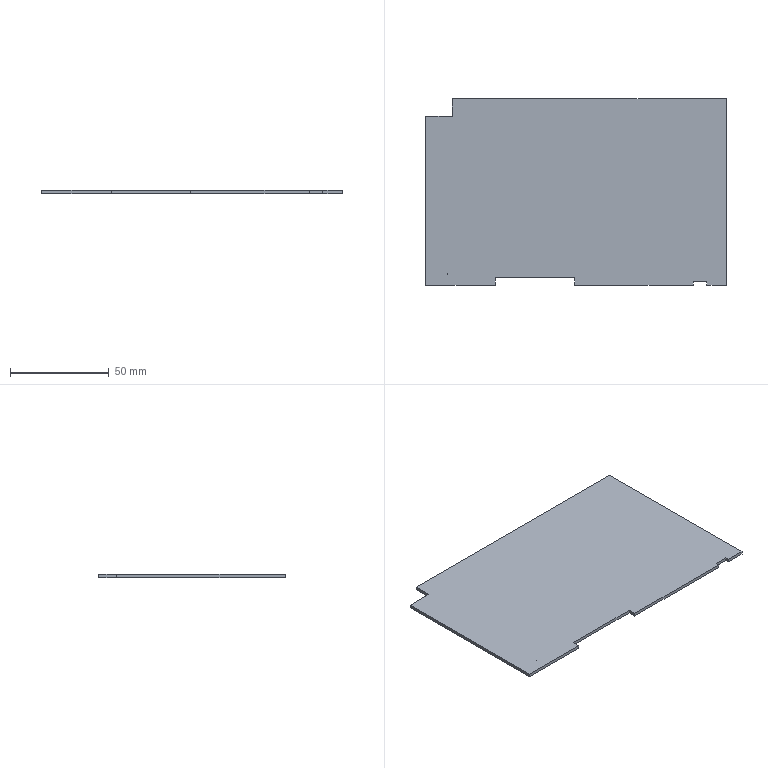Part | STEP file | LRS-150-12_X2_5F00517375-151334 | 1 solid | 18 faces | box 152 x 94.4 x 1.6 mm | volume 22494 mm3 | plane 16 | cylinder 2 | commonest cylinder face diameters 0.125 x2
STEP:
#1=CARTESIAN_POINT('',(0.,0.,0.));
#2=DIRECTION('',(0.,0.,1.));
#3=DIRECTION('',(1.,0.,0.));
#4=AXIS2_PLACEMENT_3D('',#1,#2,#3);
#5=CARTESIAN_POINT('',(-288.433,210.372,0.));
#6=VERTEX_POINT('',#5);
#7=CARTESIAN_POINT('',(-288.308,210.372,0.));
#8=VERTEX_POINT('',#7);
#9=CARTESIAN_POINT('',(-288.371,210.372,0.));
#10=DIRECTION('',(0.,0.,-1.));
#11=DIRECTION('',(-1.,0.,0.));
#12=AXIS2_PLACEMENT_3D('',#9,#10,#11);
#13=CIRCLE('',#12,0.0625);
#14=CARTESIAN_POINT('',(-288.371,210.372,-1.76));
#15=DIRECTION('',(0.,0.,1.));
#16=DIRECTION('',(-1.,0.,0.));
#17=AXIS2_PLACEMENT_3D('',#14,#15,#16);
#18=CYLINDRICAL_SURFACE('',#17,0.0625);
#19=CARTESIAN_POINT('',(6.283,1.76));
#20=DIRECTION('',(-1.,0.));
#21=VECTOR('',#20,1.);
#22=LINE('',#19,#21);
#23=(GEOMETRIC_REPRESENTATION_CONTEXT(2)PARAMETRIC_REPRESENTATION_CONTEXT()REPRESENTATION_CONTEXT('',''));
#24=DEFINITIONAL_REPRESENTATION('',(#22),#23);
#25=PCURVE('',#18,#24);
#26=CARTESIAN_POINT('',(0.,0.,0.));
#27=DIRECTION('',(0.,0.,1.));
#28=DIRECTION('',(-1.,0.,0.));
#29=AXIS2_PLACEMENT_3D('',#26,#27,#28);
#30=PLANE('',#29);
#31=CARTESIAN_POINT('',(288.433,-210.372));
#32=CARTESIAN_POINT('',(288.433,-210.481));
#33=CARTESIAN_POINT('',(288.34,-210.426));
#34=CARTESIAN_POINT('',(288.246,-210.372));
#35=CARTESIAN_POINT('',(288.34,-210.318));
#36=CARTESIAN_POINT('',(288.433,-210.264));
#37=CARTESIAN_POINT('',(288.433,-210.372));
#38=(BOUNDED_CURVE()B_SPLINE_CURVE(2,(#31,#32,#33,#34,#35,#36,#37),.UNSPECIFIED.,.T.,.F.)B_SPLINE_CURVE_WITH_KNOTS((1,2,2,2,2,1),(-2.094,0.,2.094,4.189,6.283,8.378),.UNSPECIFIED.)CURVE()GEOMETRIC_REPRESENTATION_ITEM()RATIONAL_B_SPLINE_CURVE((1.,0.5,1.,0.5,1.,0.5,1.))REPRESENTATION_ITEM(''));
#39=(GEOMETRIC_REPRESENTATION_CONTEXT(2)PARAMETRIC_REPRESENTATION_CONTEXT()REPRESENTATION_CONTEXT('',''));
#40=DEFINITIONAL_REPRESENTATION('',(#38),#39);
#41=PCURVE('',#30,#40);
#42=SURFACE_CURVE('',#13,(#25,#41),.PCURVE_S1.);
#43=EDGE_CURVE('',#6,#8,#42,.T.);
#44=ORIENTED_EDGE('',*,*,#43,.T.);
#45=CARTESIAN_POINT('',(-288.308,210.372,-1.6));
#46=VERTEX_POINT('',#45);
#47=CARTESIAN_POINT('',(-288.308,210.372,-1.6));
#48=DIRECTION('',(0.,0.,1.));
#49=VECTOR('',#48,1.);
#50=LINE('',#47,#49);
#51=CARTESIAN_POINT('',(3.142,0.16));
#52=DIRECTION('',(0.,1.));
#53=VECTOR('',#52,1.);
#54=LINE('',#51,#53);
#55=(GEOMETRIC_REPRESENTATION_CONTEXT(2)PARAMETRIC_REPRESENTATION_CONTEXT()REPRESENTATION_CONTEXT('',''));
#56=DEFINITIONAL_REPRESENTATION('',(#54),#55);
#57=PCURVE('',#18,#56);
#58=CARTESIAN_POINT('',(-288.371,210.372,-1.76));
#59=DIRECTION('',(0.,0.,1.));
#60=DIRECTION('',(-1.,0.,0.));
#61=AXIS2_PLACEMENT_3D('',#58,#59,#60);
#62=CYLINDRICAL_SURFACE('',#61,0.0625);
#63=CARTESIAN_POINT('',(3.142,0.16));
#64=DIRECTION('',(0.,1.));
#65=VECTOR('',#64,1.);
#66=LINE('',#63,#65);
#67=(GEOMETRIC_REPRESENTATION_CONTEXT(2)PARAMETRIC_REPRESENTATION_CONTEXT()REPRESENTATION_CONTEXT('',''));
#68=DEFINITIONAL_REPRESENTATION('',(#66),#67);
#69=PCURVE('',#62,#68);
#70=SURFACE_CURVE('',#50,(#57,#69),.PCURVE_S1.);
#71=EDGE_CURVE('',#46,#8,#70,.T.);
#72=ORIENTED_EDGE('',*,*,#71,.F.);
#73=CARTESIAN_POINT('',(-288.433,210.372,-1.6));
#74=VERTEX_POINT('',#73);
#75=CARTESIAN_POINT('',(-288.371,210.372,-1.6));
#76=DIRECTION('',(0.,0.,1.));
#77=DIRECTION('',(1.,0.,0.));
#78=AXIS2_PLACEMENT_3D('',#75,#76,#77);
#79=CIRCLE('',#78,0.0625);
#80=CARTESIAN_POINT('',(3.142,0.16));
#81=DIRECTION('',(1.,0.));
#82=VECTOR('',#81,1.);
#83=LINE('',#80,#82);
#84=(GEOMETRIC_REPRESENTATION_CONTEXT(2)PARAMETRIC_REPRESENTATION_CONTEXT()REPRESENTATION_CONTEXT('',''));
#85=DEFINITIONAL_REPRESENTATION('',(#83),#84);
#86=PCURVE('',#18,#85);
#87=CARTESIAN_POINT('',(0.,0.,-1.6));
#88=DIRECTION('',(0.,0.,1.));
#89=DIRECTION('',(-1.,0.,0.));
#90=AXIS2_PLACEMENT_3D('',#87,#88,#89);
#91=PLANE('',#90);
#92=CARTESIAN_POINT('',(288.371,-210.372));
#93=DIRECTION('',(-1.,0.));
#94=AXIS2_PLACEMENT_2D('',#92,#93);
#95=CIRCLE('',#94,0.0625);
#96=(GEOMETRIC_REPRESENTATION_CONTEXT(2)PARAMETRIC_REPRESENTATION_CONTEXT()REPRESENTATION_CONTEXT('',''));
#97=DEFINITIONAL_REPRESENTATION('',(#95),#96);
#98=PCURVE('',#91,#97);
#99=SURFACE_CURVE('',#79,(#86,#98),.PCURVE_S1.);
#100=EDGE_CURVE('',#46,#74,#99,.T.);
#101=ORIENTED_EDGE('',*,*,#100,.T.);
#102=CARTESIAN_POINT('',(-288.433,210.372,-1.6));
#103=DIRECTION('',(0.,0.,1.));
#104=VECTOR('',#103,1.);
#105=LINE('',#102,#104);
#106=CARTESIAN_POINT('',(6.283,0.16));
#107=DIRECTION('',(0.,1.));
#108=VECTOR('',#107,1.);
#109=LINE('',#106,#108);
#110=(GEOMETRIC_REPRESENTATION_CONTEXT(2)PARAMETRIC_REPRESENTATION_CONTEXT()REPRESENTATION_CONTEXT('',''));
#111=DEFINITIONAL_REPRESENTATION('',(#109),#110);
#112=PCURVE('',#18,#111);
#113=CARTESIAN_POINT('',(0.,0.16));
#114=DIRECTION('',(0.,1.));
#115=VECTOR('',#114,1.);
#116=LINE('',#113,#115);
#117=(GEOMETRIC_REPRESENTATION_CONTEXT(2)PARAMETRIC_REPRESENTATION_CONTEXT()REPRESENTATION_CONTEXT('',''));
#118=DEFINITIONAL_REPRESENTATION('',(#116),#117);
#119=PCURVE('',#62,#118);
#120=SURFACE_CURVE('',#105,(#112,#119),.PCURVE_S1.);
#121=EDGE_CURVE('',#74,#6,#120,.T.);
#122=ORIENTED_EDGE('',*,*,#121,.T.);
#123=EDGE_LOOP('',(#44,#72,#101,#122));
#124=FACE_BOUND('',#123,.F.);
#125=ADVANCED_FACE('',(#124),#18,.F.);
#126=CARTESIAN_POINT('',(-299.417,204.625,0.));
#127=VERTEX_POINT('',#126);
#128=CARTESIAN_POINT('',(-264.167,204.625,0.));
#129=VERTEX_POINT('',#128);
#130=CARTESIAN_POINT('',(-299.417,204.625,0.));
#131=DIRECTION('',(1.,0.,0.));
#132=VECTOR('',#131,1.);
#133=LINE('',#130,#132);
#134=CARTESIAN_POINT('',(299.417,-204.625));
#135=DIRECTION('',(-1.,0.));
#136=VECTOR('',#135,1.);
#137=LINE('',#134,#136);
#138=(GEOMETRIC_REPRESENTATION_CONTEXT(2)PARAMETRIC_REPRESENTATION_CONTEXT()REPRESENTATION_CONTEXT('',''));
#139=DEFINITIONAL_REPRESENTATION('',(#137),#138);
#140=PCURVE('',#30,#139);
#141=CARTESIAN_POINT('',(-290.417,204.625,0.));
#142=DIRECTION('',(0.,-1.,0.));
#143=DIRECTION('',(1.,0.,0.));
#144=AXIS2_PLACEMENT_3D('',#141,#142,#143);
#145=PLANE('',#144);
#146=CARTESIAN_POINT('',(-9.,0.));
#147=DIRECTION('',(1.,0.));
#148=VECTOR('',#147,1.);
#149=LINE('',#146,#148);
#150=(GEOMETRIC_REPRESENTATION_CONTEXT(2)PARAMETRIC_REPRESENTATION_CONTEXT()REPRESENTATION_CONTEXT('',''));
#151=DEFINITIONAL_REPRESENTATION('',(#149),#150);
#152=PCURVE('',#145,#151);
#153=SURFACE_CURVE('',#133,(#140,#152),.PCURVE_S1.);
#154=EDGE_CURVE('',#127,#129,#153,.T.);
#155=ORIENTED_EDGE('',*,*,#154,.F.);
#156=CARTESIAN_POINT('',(-299.417,290.025,0.));
#157=VERTEX_POINT('',#156);
#158=CARTESIAN_POINT('',(-299.417,290.025,0.));
#159=DIRECTION('',(0.,-1.,0.));
#160=VECTOR('',#159,1.);
#161=LINE('',#158,#160);
#162=CARTESIAN_POINT('',(299.417,-290.025));
#163=DIRECTION('',(0.,1.));
#164=VECTOR('',#163,1.);
#165=LINE('',#162,#164);
#166=(GEOMETRIC_REPRESENTATION_CONTEXT(2)PARAMETRIC_REPRESENTATION_CONTEXT()REPRESENTATION_CONTEXT('',''));
#167=DEFINITIONAL_REPRESENTATION('',(#165),#166);
#168=PCURVE('',#30,#167);
#169=CARTESIAN_POINT('',(-299.417,299.375,0.));
#170=DIRECTION('',(-1.,0.,0.));
#171=DIRECTION('',(0.,-1.,0.));
#172=AXIS2_PLACEMENT_3D('',#169,#170,#171);
#173=PLANE('',#172);
#174=CARTESIAN_POINT('',(9.35,0.));
#175=DIRECTION('',(1.,0.));
#176=VECTOR('',#175,1.);
#177=LINE('',#174,#176);
#178=(GEOMETRIC_REPRESENTATION_CONTEXT(2)PARAMETRIC_REPRESENTATION_CONTEXT()REPRESENTATION_CONTEXT('',''));
#179=DEFINITIONAL_REPRESENTATION('',(#177),#178);
#180=PCURVE('',#173,#179);
#181=SURFACE_CURVE('',#161,(#168,#180),.PCURVE_S1.);
#182=EDGE_CURVE('',#157,#127,#181,.T.);
#183=ORIENTED_EDGE('',*,*,#182,.F.);
#184=CARTESIAN_POINT('',(-285.934,290.025,0.));
#185=VERTEX_POINT('',#184);
#186=CARTESIAN_POINT('',(-299.417,290.025,0.));
#187=DIRECTION('',(1.,0.,0.));
#188=VECTOR('',#187,1.);
#189=LINE('',#186,#188);
#190=CARTESIAN_POINT('',(299.417,-290.025));
#191=DIRECTION('',(-1.,0.));
#192=VECTOR('',#191,1.);
#193=LINE('',#190,#192);
#194=(GEOMETRIC_REPRESENTATION_CONTEXT(2)PARAMETRIC_REPRESENTATION_CONTEXT()REPRESENTATION_CONTEXT('',''));
#195=DEFINITIONAL_REPRESENTATION('',(#193),#194);
#196=PCURVE('',#30,#195);
#197=CARTESIAN_POINT('',(-291.417,290.025,-1.76));
#198=DIRECTION('',(0.,-1.,0.));
#199=DIRECTION('',(1.,0.,0.));
#200=AXIS2_PLACEMENT_3D('',#197,#198,#199);
#201=PLANE('',#200);
#202=CARTESIAN_POINT('',(-8.,1.76));
#203=DIRECTION('',(1.,0.));
#204=VECTOR('',#203,1.);
#205=LINE('',#202,#204);
#206=(GEOMETRIC_REPRESENTATION_CONTEXT(2)PARAMETRIC_REPRESENTATION_CONTEXT()REPRESENTATION_CONTEXT('',''));
#207=DEFINITIONAL_REPRESENTATION('',(#205),#206);
#208=PCURVE('',#201,#207);
#209=SURFACE_CURVE('',#189,(#196,#208),.PCURVE_S1.);
#210=EDGE_CURVE('',#157,#185,#209,.T.);
#211=ORIENTED_EDGE('',*,*,#210,.T.);
#212=CARTESIAN_POINT('',(-285.934,299.025,0.));
#213=VERTEX_POINT('',#212);
#214=CARTESIAN_POINT('',(-285.934,299.025,0.));
#215=DIRECTION('',(0.,-1.,0.));
#216=VECTOR('',#215,1.);
#217=LINE('',#214,#216);
#218=CARTESIAN_POINT('',(285.934,-299.025));
#219=DIRECTION('',(0.,1.));
#220=VECTOR('',#219,1.);
#221=LINE('',#218,#220);
#222=(GEOMETRIC_REPRESENTATION_CONTEXT(2)PARAMETRIC_REPRESENTATION_CONTEXT()REPRESENTATION_CONTEXT('',''));
#223=DEFINITIONAL_REPRESENTATION('',(#221),#222);
#224=PCURVE('',#30,#223);
#225=CARTESIAN_POINT('',(-285.934,208.875,21.275));
#226=DIRECTION('',(-1.,0.,0.));
#227=DIRECTION('',(0.,-1.,0.));
#228=AXIS2_PLACEMENT_3D('',#225,#226,#227);
#229=PLANE('',#228);
#230=CARTESIAN_POINT('',(-90.15,-21.275));
#231=DIRECTION('',(1.,0.));
#232=VECTOR('',#231,1.);
#233=LINE('',#230,#232);
#234=(GEOMETRIC_REPRESENTATION_CONTEXT(2)PARAMETRIC_REPRESENTATION_CONTEXT()REPRESENTATION_CONTEXT('',''));
#235=DEFINITIONAL_REPRESENTATION('',(#233),#234);
#236=PCURVE('',#229,#235);
#237=SURFACE_CURVE('',#217,(#224,#236),.PCURVE_S1.);
#238=EDGE_CURVE('',#213,#185,#237,.T.);
#239=ORIENTED_EDGE('',*,*,#238,.F.);
#240=CARTESIAN_POINT('',(-147.417,299.025,0.));
#241=VERTEX_POINT('',#240);
#242=CARTESIAN_POINT('',(-147.417,299.025,0.));
#243=DIRECTION('',(-1.,0.,0.));
#244=VECTOR('',#243,1.);
#245=LINE('',#242,#244);
#246=CARTESIAN_POINT('',(147.417,-299.025));
#247=DIRECTION('',(1.,0.));
#248=VECTOR('',#247,1.);
#249=LINE('',#246,#248);
#250=(GEOMETRIC_REPRESENTATION_CONTEXT(2)PARAMETRIC_REPRESENTATION_CONTEXT()REPRESENTATION_CONTEXT('',''));
#251=DEFINITIONAL_REPRESENTATION('',(#249),#250);
#252=PCURVE('',#30,#251);
#253=CARTESIAN_POINT('',(-177.167,299.025,0.));
#254=DIRECTION('',(0.,1.,0.));
#255=DIRECTION('',(-1.,0.,0.));
#256=AXIS2_PLACEMENT_3D('',#253,#254,#255);
#257=PLANE('',#256);
#258=CARTESIAN_POINT('',(-29.75,0.));
#259=DIRECTION('',(1.,0.));
#260=VECTOR('',#259,1.);
#261=LINE('',#258,#260);
#262=(GEOMETRIC_REPRESENTATION_CONTEXT(2)PARAMETRIC_REPRESENTATION_CONTEXT()REPRESENTATION_CONTEXT('',''));
#263=DEFINITIONAL_REPRESENTATION('',(#261),#262);
#264=PCURVE('',#257,#263);
#265=SURFACE_CURVE('',#245,(#252,#264),.PCURVE_S1.);
#266=EDGE_CURVE('',#241,#213,#265,.T.);
#267=ORIENTED_EDGE('',*,*,#266,.F.);
#268=CARTESIAN_POINT('',(-147.417,204.625,0.));
#269=VERTEX_POINT('',#268);
#270=CARTESIAN_POINT('',(-147.417,204.625,0.));
#271=DIRECTION('',(0.,1.,0.));
#272=VECTOR('',#271,1.);
#273=LINE('',#270,#272);
#274=CARTESIAN_POINT('',(147.417,-204.625));
#275=DIRECTION('',(0.,-1.));
#276=VECTOR('',#275,1.);
#277=LINE('',#274,#276);
#278=(GEOMETRIC_REPRESENTATION_CONTEXT(2)PARAMETRIC_REPRESENTATION_CONTEXT()REPRESENTATION_CONTEXT('',''));
#279=DEFINITIONAL_REPRESENTATION('',(#277),#278);
#280=PCURVE('',#30,#279);
#281=CARTESIAN_POINT('',(-147.417,204.625,0.));
#282=DIRECTION('',(1.,0.,0.));
#283=DIRECTION('',(0.,1.,0.));
#284=AXIS2_PLACEMENT_3D('',#281,#282,#283);
#285=PLANE('',#284);
#286=CARTESIAN_POINT('',(0.,0.));
#287=DIRECTION('',(1.,0.));
#288=VECTOR('',#287,1.);
#289=LINE('',#286,#288);
#290=(GEOMETRIC_REPRESENTATION_CONTEXT(2)PARAMETRIC_REPRESENTATION_CONTEXT()REPRESENTATION_CONTEXT('',''));
#291=DEFINITIONAL_REPRESENTATION('',(#289),#290);
#292=PCURVE('',#285,#291);
#293=SURFACE_CURVE('',#273,(#280,#292),.PCURVE_S1.);
#294=EDGE_CURVE('',#269,#241,#293,.T.);
#295=ORIENTED_EDGE('',*,*,#294,.F.);
#296=CARTESIAN_POINT('',(-157.222,204.625,0.));
#297=VERTEX_POINT('',#296);
#298=CARTESIAN_POINT('',(-157.222,204.625,0.));
#299=DIRECTION('',(1.,0.,0.));
#300=VECTOR('',#299,1.);
#301=LINE('',#298,#300);
#302=CARTESIAN_POINT('',(157.222,-204.625));
#303=DIRECTION('',(-1.,0.));
#304=VECTOR('',#303,1.);
#305=LINE('',#302,#304);
#306=(GEOMETRIC_REPRESENTATION_CONTEXT(2)PARAMETRIC_REPRESENTATION_CONTEXT()REPRESENTATION_CONTEXT('',''));
#307=DEFINITIONAL_REPRESENTATION('',(#305),#306);
#308=PCURVE('',#30,#307);
#309=CARTESIAN_POINT('',(-320.417,204.625,0.));
#310=DIRECTION('',(0.,-1.,0.));
#311=DIRECTION('',(1.,0.,0.));
#312=AXIS2_PLACEMENT_3D('',#309,#310,#311);
#313=PLANE('',#312);
#314=CARTESIAN_POINT('',(163.195,0.));
#315=DIRECTION('',(1.,0.));
#316=VECTOR('',#315,1.);
#317=LINE('',#314,#316);
#318=(GEOMETRIC_REPRESENTATION_CONTEXT(2)PARAMETRIC_REPRESENTATION_CONTEXT()REPRESENTATION_CONTEXT('',''));
#319=DEFINITIONAL_REPRESENTATION('',(#317),#318);
#320=PCURVE('',#313,#319);
#321=SURFACE_CURVE('',#301,(#308,#320),.PCURVE_S1.);
#322=EDGE_CURVE('',#297,#269,#321,.T.);
#323=ORIENTED_EDGE('',*,*,#322,.F.);
#324=CARTESIAN_POINT('',(-157.222,206.435,0.));
#325=VERTEX_POINT('',#324);
#326=CARTESIAN_POINT('',(-157.222,204.625,0.));
#327=DIRECTION('',(0.,1.,0.));
#328=VECTOR('',#327,1.);
#329=LINE('',#326,#328);
#330=CARTESIAN_POINT('',(157.222,-204.625));
#331=DIRECTION('',(0.,-1.));
#332=VECTOR('',#331,1.);
#333=LINE('',#330,#332);
#334=(GEOMETRIC_REPRESENTATION_CONTEXT(2)PARAMETRIC_REPRESENTATION_CONTEXT()REPRESENTATION_CONTEXT('',''));
#335=DEFINITIONAL_REPRESENTATION('',(#333),#334);
#336=PCURVE('',#30,#335);
#337=CARTESIAN_POINT('',(-157.222,205.935,-1.76));
#338=DIRECTION('',(1.,0.,0.));
#339=DIRECTION('',(0.,1.,0.));
#340=AXIS2_PLACEMENT_3D('',#337,#338,#339);
#341=PLANE('',#340);
#342=CARTESIAN_POINT('',(-1.31,1.76));
#343=DIRECTION('',(1.,0.));
#344=VECTOR('',#343,1.);
#345=LINE('',#342,#344);
#346=(GEOMETRIC_REPRESENTATION_CONTEXT(2)PARAMETRIC_REPRESENTATION_CONTEXT()REPRESENTATION_CONTEXT('',''));
#347=DEFINITIONAL_REPRESENTATION('',(#345),#346);
#348=PCURVE('',#341,#347);
#349=SURFACE_CURVE('',#329,(#336,#348),.PCURVE_S1.);
#350=EDGE_CURVE('',#297,#325,#349,.T.);
#351=ORIENTED_EDGE('',*,*,#350,.T.);
#352=CARTESIAN_POINT('',(-164.112,206.435,0.));
#353=VERTEX_POINT('',#352);
#354=CARTESIAN_POINT('',(-157.222,206.435,0.));
#355=DIRECTION('',(-1.,0.,0.));
#356=VECTOR('',#355,1.);
#357=LINE('',#354,#356);
#358=CARTESIAN_POINT('',(157.222,-206.435));
#359=DIRECTION('',(1.,0.));
#360=VECTOR('',#359,1.);
#361=LINE('',#358,#360);
#362=(GEOMETRIC_REPRESENTATION_CONTEXT(2)PARAMETRIC_REPRESENTATION_CONTEXT()REPRESENTATION_CONTEXT('',''));
#363=DEFINITIONAL_REPRESENTATION('',(#361),#362);
#364=PCURVE('',#30,#363);
#365=CARTESIAN_POINT('',(-164.112,206.435,-1.76));
#366=DIRECTION('',(0.,1.,0.));
#367=DIRECTION('',(-1.,0.,0.));
#368=AXIS2_PLACEMENT_3D('',#365,#366,#367);
#369=PLANE('',#368);
#370=CARTESIAN_POINT('',(-6.89,1.76));
#371=DIRECTION('',(1.,0.));
#372=VECTOR('',#371,1.);
#373=LINE('',#370,#372);
#374=(GEOMETRIC_REPRESENTATION_CONTEXT(2)PARAMETRIC_REPRESENTATION_CONTEXT()REPRESENTATION_CONTEXT('',''));
#375=DEFINITIONAL_REPRESENTATION('',(#373),#374);
#376=PCURVE('',#369,#375);
#377=SURFACE_CURVE('',#357,(#364,#376),.PCURVE_S1.);
#378=EDGE_CURVE('',#325,#353,#377,.T.);
#379=ORIENTED_EDGE('',*,*,#378,.T.);
#380=CARTESIAN_POINT('',(-164.112,204.625,0.));
#381=VERTEX_POINT('',#380);
#382=CARTESIAN_POINT('',(-164.112,206.435,0.));
#383=DIRECTION('',(0.,-1.,0.));
#384=VECTOR('',#383,1.);
#385=LINE('',#382,#384);
#386=CARTESIAN_POINT('',(164.112,-206.435));
#387=DIRECTION('',(0.,1.));
#388=VECTOR('',#387,1.);
#389=LINE('',#386,#388);
#390=(GEOMETRIC_REPRESENTATION_CONTEXT(2)PARAMETRIC_REPRESENTATION_CONTEXT()REPRESENTATION_CONTEXT('',''));
#391=DEFINITIONAL_REPRESENTATION('',(#389),#390);
#392=PCURVE('',#30,#391);
#393=CARTESIAN_POINT('',(-164.112,200.574,-1.76));
#394=DIRECTION('',(-1.,0.,0.));
#395=DIRECTION('',(0.,-1.,0.));
#396=AXIS2_PLACEMENT_3D('',#393,#394,#395);
#397=PLANE('',#396);
#398=CARTESIAN_POINT('',(-5.861,1.76));
#399=DIRECTION('',(1.,0.));
#400=VECTOR('',#399,1.);
#401=LINE('',#398,#400);
#402=(GEOMETRIC_REPRESENTATION_CONTEXT(2)PARAMETRIC_REPRESENTATION_CONTEXT()REPRESENTATION_CONTEXT('',''));
#403=DEFINITIONAL_REPRESENTATION('',(#401),#402);
#404=PCURVE('',#397,#403);
#405=SURFACE_CURVE('',#385,(#392,#404),.PCURVE_S1.);
#406=EDGE_CURVE('',#353,#381,#405,.T.);
#407=ORIENTED_EDGE('',*,*,#406,.T.);
#408=CARTESIAN_POINT('',(-224.167,204.625,0.));
#409=VERTEX_POINT('',#408);
#410=CARTESIAN_POINT('',(-224.167,204.625,0.));
#411=DIRECTION('',(1.,0.,0.));
#412=VECTOR('',#411,1.);
#413=LINE('',#410,#412);
#414=CARTESIAN_POINT('',(224.167,-204.625));
#415=DIRECTION('',(-1.,0.));
#416=VECTOR('',#415,1.);
#417=LINE('',#414,#416);
#418=(GEOMETRIC_REPRESENTATION_CONTEXT(2)PARAMETRIC_REPRESENTATION_CONTEXT()REPRESENTATION_CONTEXT('',''));
#419=DEFINITIONAL_REPRESENTATION('',(#417),#418);
#420=PCURVE('',#30,#419);
#421=CARTESIAN_POINT('',(-320.417,204.625,0.));
#422=DIRECTION('',(0.,-1.,0.));
#423=DIRECTION('',(1.,0.,0.));
#424=AXIS2_PLACEMENT_3D('',#421,#422,#423);
#425=PLANE('',#424);
#426=CARTESIAN_POINT('',(96.25,0.));
#427=DIRECTION('',(1.,0.));
#428=VECTOR('',#427,1.);
#429=LINE('',#426,#428);
#430=(GEOMETRIC_REPRESENTATION_CONTEXT(2)PARAMETRIC_REPRESENTATION_CONTEXT()REPRESENTATION_CONTEXT('',''));
#431=DEFINITIONAL_REPRESENTATION('',(#429),#430);
#432=PCURVE('',#425,#431);
#433=SURFACE_CURVE('',#413,(#420,#432),.PCURVE_S1.);
#434=EDGE_CURVE('',#409,#381,#433,.T.);
#435=ORIENTED_EDGE('',*,*,#434,.F.);
#436=CARTESIAN_POINT('',(-224.167,208.525,0.));
#437=VERTEX_POINT('',#436);
#438=CARTESIAN_POINT('',(-224.167,204.625,0.));
#439=DIRECTION('',(0.,1.,0.));
#440=VECTOR('',#439,1.);
#441=LINE('',#438,#440);
#442=CARTESIAN_POINT('',(224.167,-204.625));
#443=DIRECTION('',(0.,-1.));
#444=VECTOR('',#443,1.);
#445=LINE('',#442,#444);
#446=(GEOMETRIC_REPRESENTATION_CONTEXT(2)PARAMETRIC_REPRESENTATION_CONTEXT()REPRESENTATION_CONTEXT('',''));
#447=DEFINITIONAL_REPRESENTATION('',(#445),#446);
#448=PCURVE('',#30,#447);
#449=CARTESIAN_POINT('',(-224.167,208.775,-1.76));
#450=DIRECTION('',(1.,0.,0.));
#451=DIRECTION('',(0.,1.,0.));
#452=AXIS2_PLACEMENT_3D('',#449,#450,#451);
#453=PLANE('',#452);
#454=CARTESIAN_POINT('',(-4.15,1.76));
#455=DIRECTION('',(1.,0.));
#456=VECTOR('',#455,1.);
#457=LINE('',#454,#456);
#458=(GEOMETRIC_REPRESENTATION_CONTEXT(2)PARAMETRIC_REPRESENTATION_CONTEXT()REPRESENTATION_CONTEXT('',''));
#459=DEFINITIONAL_REPRESENTATION('',(#457),#458);
#460=PCURVE('',#453,#459);
#461=SURFACE_CURVE('',#441,(#448,#460),.PCURVE_S1.);
#462=EDGE_CURVE('',#409,#437,#461,.T.);
#463=ORIENTED_EDGE('',*,*,#462,.T.);
#464=CARTESIAN_POINT('',(-264.167,208.525,0.));
#465=VERTEX_POINT('',#464);
#466=CARTESIAN_POINT('',(-224.167,208.525,0.));
#467=DIRECTION('',(-1.,0.,0.));
#468=VECTOR('',#467,1.);
#469=LINE('',#466,#468);
#470=CARTESIAN_POINT('',(224.167,-208.525));
#471=DIRECTION('',(1.,0.));
#472=VECTOR('',#471,1.);
#473=LINE('',#470,#472);
#474=(GEOMETRIC_REPRESENTATION_CONTEXT(2)PARAMETRIC_REPRESENTATION_CONTEXT()REPRESENTATION_CONTEXT('',''));
#475=DEFINITIONAL_REPRESENTATION('',(#473),#474);
#476=PCURVE('',#30,#475);
#477=CARTESIAN_POINT('',(-260.592,208.525,-1.76));
#478=DIRECTION('',(0.,1.,0.));
#479=DIRECTION('',(-1.,0.,0.));
#480=AXIS2_PLACEMENT_3D('',#477,#478,#479);
#481=PLANE('',#480);
#482=CARTESIAN_POINT('',(-36.425,1.76));
#483=DIRECTION('',(1.,0.));
#484=VECTOR('',#483,1.);
#485=LINE('',#482,#484);
#486=(GEOMETRIC_REPRESENTATION_CONTEXT(2)PARAMETRIC_REPRESENTATION_CONTEXT()REPRESENTATION_CONTEXT('',''));
#487=DEFINITIONAL_REPRESENTATION('',(#485),#486);
#488=PCURVE('',#481,#487);
#489=SURFACE_CURVE('',#469,(#476,#488),.PCURVE_S1.);
#490=EDGE_CURVE('',#437,#465,#489,.T.);
#491=ORIENTED_EDGE('',*,*,#490,.T.);
#492=CARTESIAN_POINT('',(-264.167,208.525,0.));
#493=DIRECTION('',(0.,-1.,0.));
#494=VECTOR('',#493,1.);
#495=LINE('',#492,#494);
#496=CARTESIAN_POINT('',(264.167,-208.525));
#497=DIRECTION('',(0.,1.));
#498=VECTOR('',#497,1.);
#499=LINE('',#496,#498);
#500=(GEOMETRIC_REPRESENTATION_CONTEXT(2)PARAMETRIC_REPRESENTATION_CONTEXT()REPRESENTATION_CONTEXT('',''));
#501=DEFINITIONAL_REPRESENTATION('',(#499),#500);
#502=PCURVE('',#30,#501);
#503=CARTESIAN_POINT('',(-264.167,199.339,-1.76));
#504=DIRECTION('',(-1.,0.,0.));
#505=DIRECTION('',(0.,-1.,0.));
#506=AXIS2_PLACEMENT_3D('',#503,#504,#505);
#507=PLANE('',#506);
#508=CARTESIAN_POINT('',(-9.185,1.76));
#509=DIRECTION('',(1.,0.));
#510=VECTOR('',#509,1.);
#511=LINE('',#508,#510);
#512=(GEOMETRIC_REPRESENTATION_CONTEXT(2)PARAMETRIC_REPRESENTATION_CONTEXT()REPRESENTATION_CONTEXT('',''));
#513=DEFINITIONAL_REPRESENTATION('',(#511),#512);
#514=PCURVE('',#507,#513);
#515=SURFACE_CURVE('',#495,(#502,#514),.PCURVE_S1.);
#516=EDGE_CURVE('',#465,#129,#515,.T.);
#517=ORIENTED_EDGE('',*,*,#516,.T.);
#518=EDGE_LOOP('',(#155,#183,#211,#239,#267,#295,#323,#351,#379,#407,#435,#463,#491,#517));
#519=FACE_BOUND('',#518,.F.);
#520=ORIENTED_EDGE('',*,*,#43,.F.);
#521=CARTESIAN_POINT('',(-288.371,210.372,0.));
#522=DIRECTION('',(0.,0.,-1.));
#523=DIRECTION('',(1.,0.,0.));
#524=AXIS2_PLACEMENT_3D('',#521,#522,#523);
#525=CIRCLE('',#524,0.0625);
#526=CARTESIAN_POINT('',(288.308,-210.372));
#527=CARTESIAN_POINT('',(288.308,-210.264));
#528=CARTESIAN_POINT('',(288.402,-210.318));
#529=CARTESIAN_POINT('',(288.496,-210.372));
#530=CARTESIAN_POINT('',(288.402,-210.426));
#531=CARTESIAN_POINT('',(288.308,-210.481));
#532=CARTESIAN_POINT('',(288.308,-210.372));
#533=(BOUNDED_CURVE()B_SPLINE_CURVE(2,(#526,#527,#528,#529,#530,#531,#532),.UNSPECIFIED.,.T.,.F.)B_SPLINE_CURVE_WITH_KNOTS((1,2,2,2,2,1),(-2.094,0.,2.094,4.189,6.283,8.378),.UNSPECIFIED.)CURVE()GEOMETRIC_REPRESENTATION_ITEM()RATIONAL_B_SPLINE_CURVE((1.,0.5,1.,0.5,1.,0.5,1.))REPRESENTATION_ITEM(''));
#534=(GEOMETRIC_REPRESENTATION_CONTEXT(2)PARAMETRIC_REPRESENTATION_CONTEXT()REPRESENTATION_CONTEXT('',''));
#535=DEFINITIONAL_REPRESENTATION('',(#533),#534);
#536=PCURVE('',#30,#535);
#537=CARTESIAN_POINT('',(3.142,1.76));
#538=DIRECTION('',(-1.,0.));
#539=VECTOR('',#538,1.);
#540=LINE('',#537,#539);
#541=(GEOMETRIC_REPRESENTATION_CONTEXT(2)PARAMETRIC_REPRESENTATION_CONTEXT()REPRESENTATION_CONTEXT('',''));
#542=DEFINITIONAL_REPRESENTATION('',(#540),#541);
#543=PCURVE('',#62,#542);
#544=SURFACE_CURVE('',#525,(#536,#543),.PCURVE_S1.);
#545=EDGE_CURVE('',#8,#6,#544,.T.);
#546=ORIENTED_EDGE('',*,*,#545,.F.);
#547=EDGE_LOOP('',(#520,#546));
#548=FACE_BOUND('',#547,.F.);
#549=ADVANCED_FACE('',(#519,#548),#30,.T.);
#550=ORIENTED_EDGE('',*,*,#71,.T.);
#551=ORIENTED_EDGE('',*,*,#545,.T.);
#552=ORIENTED_EDGE('',*,*,#121,.F.);
#553=CARTESIAN_POINT('',(-288.371,210.372,-1.6));
#554=DIRECTION('',(0.,0.,1.));
#555=DIRECTION('',(-1.,0.,0.));
#556=AXIS2_PLACEMENT_3D('',#553,#554,#555);
#557=CIRCLE('',#556,0.0625);
#558=CARTESIAN_POINT('',(0.,0.16));
#559=DIRECTION('',(1.,0.));
#560=VECTOR('',#559,1.);
#561=LINE('',#558,#560);
#562=(GEOMETRIC_REPRESENTATION_CONTEXT(2)PARAMETRIC_REPRESENTATION_CONTEXT()REPRESENTATION_CONTEXT('',''));
#563=DEFINITIONAL_REPRESENTATION('',(#561),#562);
#564=PCURVE('',#62,#563);
#565=CARTESIAN_POINT('',(288.371,-210.372));
#566=DIRECTION('',(1.,0.));
#567=AXIS2_PLACEMENT_2D('',#565,#566);
#568=CIRCLE('',#567,0.0625);
#569=(GEOMETRIC_REPRESENTATION_CONTEXT(2)PARAMETRIC_REPRESENTATION_CONTEXT()REPRESENTATION_CONTEXT('',''));
#570=DEFINITIONAL_REPRESENTATION('',(#568),#569);
#571=PCURVE('',#91,#570);
#572=SURFACE_CURVE('',#557,(#564,#571),.PCURVE_S1.);
#573=EDGE_CURVE('',#74,#46,#572,.T.);
#574=ORIENTED_EDGE('',*,*,#573,.T.);
#575=EDGE_LOOP('',(#550,#551,#552,#574));
#576=FACE_BOUND('',#575,.F.);
#577=ADVANCED_FACE('',(#576),#62,.F.);
#578=CARTESIAN_POINT('',(-285.934,299.025,-1.6));
#579=VERTEX_POINT('',#578);
#580=CARTESIAN_POINT('',(-285.934,290.025,-1.6));
#581=VERTEX_POINT('',#580);
#582=CARTESIAN_POINT('',(-285.934,299.025,-1.6));
#583=DIRECTION('',(0.,-1.,0.));
#584=VECTOR('',#583,1.);
#585=LINE('',#582,#584);
#586=CARTESIAN_POINT('',(285.934,-299.025));
#587=DIRECTION('',(0.,1.));
#588=VECTOR('',#587,1.);
#589=LINE('',#586,#588);
#590=(GEOMETRIC_REPRESENTATION_CONTEXT(2)PARAMETRIC_REPRESENTATION_CONTEXT()REPRESENTATION_CONTEXT('',''));
#591=DEFINITIONAL_REPRESENTATION('',(#589),#590);
#592=PCURVE('',#91,#591);
#593=CARTESIAN_POINT('',(-90.15,-22.875));
#594=DIRECTION('',(1.,0.));
#595=VECTOR('',#594,1.);
#596=LINE('',#593,#595);
#597=(GEOMETRIC_REPRESENTATION_CONTEXT(2)PARAMETRIC_REPRESENTATION_CONTEXT()REPRESENTATION_CONTEXT('',''));
#598=DEFINITIONAL_REPRESENTATION('',(#596),#597);
#599=PCURVE('',#229,#598);
#600=SURFACE_CURVE('',#585,(#592,#599),.PCURVE_S1.);
#601=EDGE_CURVE('',#579,#581,#600,.T.);
#602=ORIENTED_EDGE('',*,*,#601,.T.);
#603=CARTESIAN_POINT('',(-299.417,290.025,-1.6));
#604=VERTEX_POINT('',#603);
#605=CARTESIAN_POINT('',(-299.417,290.025,-1.6));
#606=DIRECTION('',(1.,0.,0.));
#607=VECTOR('',#606,1.);
#608=LINE('',#605,#607);
#609=CARTESIAN_POINT('',(299.417,-290.025));
#610=DIRECTION('',(-1.,0.));
#611=VECTOR('',#610,1.);
#612=LINE('',#609,#611);
#613=(GEOMETRIC_REPRESENTATION_CONTEXT(2)PARAMETRIC_REPRESENTATION_CONTEXT()REPRESENTATION_CONTEXT('',''));
#614=DEFINITIONAL_REPRESENTATION('',(#612),#613);
#615=PCURVE('',#91,#614);
#616=CARTESIAN_POINT('',(-8.,0.16));
#617=DIRECTION('',(1.,0.));
#618=VECTOR('',#617,1.);
#619=LINE('',#616,#618);
#620=(GEOMETRIC_REPRESENTATION_CONTEXT(2)PARAMETRIC_REPRESENTATION_CONTEXT()REPRESENTATION_CONTEXT('',''));
#621=DEFINITIONAL_REPRESENTATION('',(#619),#620);
#622=PCURVE('',#201,#621);
#623=SURFACE_CURVE('',#608,(#615,#622),.PCURVE_S1.);
#624=EDGE_CURVE('',#604,#581,#623,.T.);
#625=ORIENTED_EDGE('',*,*,#624,.F.);
#626=CARTESIAN_POINT('',(-299.417,204.625,-1.6));
#627=VERTEX_POINT('',#626);
#628=CARTESIAN_POINT('',(-299.417,290.025,-1.6));
#629=DIRECTION('',(0.,-1.,0.));
#630=VECTOR('',#629,1.);
#631=LINE('',#628,#630);
#632=CARTESIAN_POINT('',(299.417,-290.025));
#633=DIRECTION('',(0.,1.));
#634=VECTOR('',#633,1.);
#635=LINE('',#632,#634);
#636=(GEOMETRIC_REPRESENTATION_CONTEXT(2)PARAMETRIC_REPRESENTATION_CONTEXT()REPRESENTATION_CONTEXT('',''));
#637=DEFINITIONAL_REPRESENTATION('',(#635),#636);
#638=PCURVE('',#91,#637);
#639=CARTESIAN_POINT('',(9.35,-1.6));
#640=DIRECTION('',(1.,0.));
#641=VECTOR('',#640,1.);
#642=LINE('',#639,#641);
#643=(GEOMETRIC_REPRESENTATION_CONTEXT(2)PARAMETRIC_REPRESENTATION_CONTEXT()REPRESENTATION_CONTEXT('',''));
#644=DEFINITIONAL_REPRESENTATION('',(#642),#643);
#645=PCURVE('',#173,#644);
#646=SURFACE_CURVE('',#631,(#638,#645),.PCURVE_S1.);
#647=EDGE_CURVE('',#604,#627,#646,.T.);
#648=ORIENTED_EDGE('',*,*,#647,.T.);
#649=CARTESIAN_POINT('',(-264.167,204.625,-1.6));
#650=VERTEX_POINT('',#649);
#651=CARTESIAN_POINT('',(-299.417,204.625,-1.6));
#652=DIRECTION('',(1.,0.,0.));
#653=VECTOR('',#652,1.);
#654=LINE('',#651,#653);
#655=CARTESIAN_POINT('',(299.417,-204.625));
#656=DIRECTION('',(-1.,0.));
#657=VECTOR('',#656,1.);
#658=LINE('',#655,#657);
#659=(GEOMETRIC_REPRESENTATION_CONTEXT(2)PARAMETRIC_REPRESENTATION_CONTEXT()REPRESENTATION_CONTEXT('',''));
#660=DEFINITIONAL_REPRESENTATION('',(#658),#659);
#661=PCURVE('',#91,#660);
#662=CARTESIAN_POINT('',(-9.,-1.6));
#663=DIRECTION('',(1.,0.));
#664=VECTOR('',#663,1.);
#665=LINE('',#662,#664);
#666=(GEOMETRIC_REPRESENTATION_CONTEXT(2)PARAMETRIC_REPRESENTATION_CONTEXT()REPRESENTATION_CONTEXT('',''));
#667=DEFINITIONAL_REPRESENTATION('',(#665),#666);
#668=PCURVE('',#145,#667);
#669=SURFACE_CURVE('',#654,(#661,#668),.PCURVE_S1.);
#670=EDGE_CURVE('',#627,#650,#669,.T.);
#671=ORIENTED_EDGE('',*,*,#670,.T.);
#672=CARTESIAN_POINT('',(-264.167,208.525,-1.6));
#673=VERTEX_POINT('',#672);
#674=CARTESIAN_POINT('',(-264.167,208.525,-1.6));
#675=DIRECTION('',(0.,-1.,0.));
#676=VECTOR('',#675,1.);
#677=LINE('',#674,#676);
#678=CARTESIAN_POINT('',(264.167,-208.525));
#679=DIRECTION('',(0.,1.));
#680=VECTOR('',#679,1.);
#681=LINE('',#678,#680);
#682=(GEOMETRIC_REPRESENTATION_CONTEXT(2)PARAMETRIC_REPRESENTATION_CONTEXT()REPRESENTATION_CONTEXT('',''));
#683=DEFINITIONAL_REPRESENTATION('',(#681),#682);
#684=PCURVE('',#91,#683);
#685=CARTESIAN_POINT('',(-9.185,0.16));
#686=DIRECTION('',(1.,0.));
#687=VECTOR('',#686,1.);
#688=LINE('',#685,#687);
#689=(GEOMETRIC_REPRESENTATION_CONTEXT(2)PARAMETRIC_REPRESENTATION_CONTEXT()REPRESENTATION_CONTEXT('',''));
#690=DEFINITIONAL_REPRESENTATION('',(#688),#689);
#691=PCURVE('',#507,#690);
#692=SURFACE_CURVE('',#677,(#684,#691),.PCURVE_S1.);
#693=EDGE_CURVE('',#673,#650,#692,.T.);
#694=ORIENTED_EDGE('',*,*,#693,.F.);
#695=CARTESIAN_POINT('',(-224.167,208.525,-1.6));
#696=VERTEX_POINT('',#695);
#697=CARTESIAN_POINT('',(-224.167,208.525,-1.6));
#698=DIRECTION('',(-1.,0.,0.));
#699=VECTOR('',#698,1.);
#700=LINE('',#697,#699);
#701=CARTESIAN_POINT('',(224.167,-208.525));
#702=DIRECTION('',(1.,0.));
#703=VECTOR('',#702,1.);
#704=LINE('',#701,#703);
#705=(GEOMETRIC_REPRESENTATION_CONTEXT(2)PARAMETRIC_REPRESENTATION_CONTEXT()REPRESENTATION_CONTEXT('',''));
#706=DEFINITIONAL_REPRESENTATION('',(#704),#705);
#707=PCURVE('',#91,#706);
#708=CARTESIAN_POINT('',(-36.425,0.16));
#709=DIRECTION('',(1.,0.));
#710=VECTOR('',#709,1.);
#711=LINE('',#708,#710);
#712=(GEOMETRIC_REPRESENTATION_CONTEXT(2)PARAMETRIC_REPRESENTATION_CONTEXT()REPRESENTATION_CONTEXT('',''));
#713=DEFINITIONAL_REPRESENTATION('',(#711),#712);
#714=PCURVE('',#481,#713);
#715=SURFACE_CURVE('',#700,(#707,#714),.PCURVE_S1.);
#716=EDGE_CURVE('',#696,#673,#715,.T.);
#717=ORIENTED_EDGE('',*,*,#716,.F.);
#718=CARTESIAN_POINT('',(-224.167,204.625,-1.6));
#719=VERTEX_POINT('',#718);
#720=CARTESIAN_POINT('',(-224.167,204.625,-1.6));
#721=DIRECTION('',(0.,1.,0.));
#722=VECTOR('',#721,1.);
#723=LINE('',#720,#722);
#724=CARTESIAN_POINT('',(224.167,-204.625));
#725=DIRECTION('',(0.,-1.));
#726=VECTOR('',#725,1.);
#727=LINE('',#724,#726);
#728=(GEOMETRIC_REPRESENTATION_CONTEXT(2)PARAMETRIC_REPRESENTATION_CONTEXT()REPRESENTATION_CONTEXT('',''));
#729=DEFINITIONAL_REPRESENTATION('',(#727),#728);
#730=PCURVE('',#91,#729);
#731=CARTESIAN_POINT('',(-4.15,0.16));
#732=DIRECTION('',(1.,0.));
#733=VECTOR('',#732,1.);
#734=LINE('',#731,#733);
#735=(GEOMETRIC_REPRESENTATION_CONTEXT(2)PARAMETRIC_REPRESENTATION_CONTEXT()REPRESENTATION_CONTEXT('',''));
#736=DEFINITIONAL_REPRESENTATION('',(#734),#735);
#737=PCURVE('',#453,#736);
#738=SURFACE_CURVE('',#723,(#730,#737),.PCURVE_S1.);
#739=EDGE_CURVE('',#719,#696,#738,.T.);
#740=ORIENTED_EDGE('',*,*,#739,.F.);
#741=CARTESIAN_POINT('',(-164.112,204.625,-1.6));
#742=VERTEX_POINT('',#741);
#743=CARTESIAN_POINT('',(-224.167,204.625,-1.6));
#744=DIRECTION('',(1.,0.,0.));
#745=VECTOR('',#744,1.);
#746=LINE('',#743,#745);
#747=CARTESIAN_POINT('',(224.167,-204.625));
#748=DIRECTION('',(-1.,0.));
#749=VECTOR('',#748,1.);
#750=LINE('',#747,#749);
#751=(GEOMETRIC_REPRESENTATION_CONTEXT(2)PARAMETRIC_REPRESENTATION_CONTEXT()REPRESENTATION_CONTEXT('',''));
#752=DEFINITIONAL_REPRESENTATION('',(#750),#751);
#753=PCURVE('',#91,#752);
#754=CARTESIAN_POINT('',(96.25,-1.6));
#755=DIRECTION('',(1.,0.));
#756=VECTOR('',#755,1.);
#757=LINE('',#754,#756);
#758=(GEOMETRIC_REPRESENTATION_CONTEXT(2)PARAMETRIC_REPRESENTATION_CONTEXT()REPRESENTATION_CONTEXT('',''));
#759=DEFINITIONAL_REPRESENTATION('',(#757),#758);
#760=PCURVE('',#425,#759);
#761=SURFACE_CURVE('',#746,(#753,#760),.PCURVE_S1.);
#762=EDGE_CURVE('',#719,#742,#761,.T.);
#763=ORIENTED_EDGE('',*,*,#762,.T.);
#764=CARTESIAN_POINT('',(-164.112,206.435,-1.6));
#765=VERTEX_POINT('',#764);
#766=CARTESIAN_POINT('',(-164.112,206.435,-1.6));
#767=DIRECTION('',(0.,-1.,0.));
#768=VECTOR('',#767,1.);
#769=LINE('',#766,#768);
#770=CARTESIAN_POINT('',(164.112,-206.435));
#771=DIRECTION('',(0.,1.));
#772=VECTOR('',#771,1.);
#773=LINE('',#770,#772);
#774=(GEOMETRIC_REPRESENTATION_CONTEXT(2)PARAMETRIC_REPRESENTATION_CONTEXT()REPRESENTATION_CONTEXT('',''));
#775=DEFINITIONAL_REPRESENTATION('',(#773),#774);
#776=PCURVE('',#91,#775);
#777=CARTESIAN_POINT('',(-5.861,0.16));
#778=DIRECTION('',(1.,0.));
#779=VECTOR('',#778,1.);
#780=LINE('',#777,#779);
#781=(GEOMETRIC_REPRESENTATION_CONTEXT(2)PARAMETRIC_REPRESENTATION_CONTEXT()REPRESENTATION_CONTEXT('',''));
#782=DEFINITIONAL_REPRESENTATION('',(#780),#781);
#783=PCURVE('',#397,#782);
#784=SURFACE_CURVE('',#769,(#776,#783),.PCURVE_S1.);
#785=EDGE_CURVE('',#765,#742,#784,.T.);
#786=ORIENTED_EDGE('',*,*,#785,.F.);
#787=CARTESIAN_POINT('',(-157.222,206.435,-1.6));
#788=VERTEX_POINT('',#787);
#789=CARTESIAN_POINT('',(-157.222,206.435,-1.6));
#790=DIRECTION('',(-1.,0.,0.));
#791=VECTOR('',#790,1.);
#792=LINE('',#789,#791);
#793=CARTESIAN_POINT('',(157.222,-206.435));
#794=DIRECTION('',(1.,0.));
#795=VECTOR('',#794,1.);
#796=LINE('',#793,#795);
#797=(GEOMETRIC_REPRESENTATION_CONTEXT(2)PARAMETRIC_REPRESENTATION_CONTEXT()REPRESENTATION_CONTEXT('',''));
#798=DEFINITIONAL_REPRESENTATION('',(#796),#797);
#799=PCURVE('',#91,#798);
#800=CARTESIAN_POINT('',(-6.89,0.16));
#801=DIRECTION('',(1.,0.));
#802=VECTOR('',#801,1.);
#803=LINE('',#800,#802);
#804=(GEOMETRIC_REPRESENTATION_CONTEXT(2)PARAMETRIC_REPRESENTATION_CONTEXT()REPRESENTATION_CONTEXT('',''));
#805=DEFINITIONAL_REPRESENTATION('',(#803),#804);
#806=PCURVE('',#369,#805);
#807=SURFACE_CURVE('',#792,(#799,#806),.PCURVE_S1.);
#808=EDGE_CURVE('',#788,#765,#807,.T.);
#809=ORIENTED_EDGE('',*,*,#808,.F.);
#810=CARTESIAN_POINT('',(-157.222,204.625,-1.6));
#811=VERTEX_POINT('',#810);
#812=CARTESIAN_POINT('',(-157.222,204.625,-1.6));
#813=DIRECTION('',(0.,1.,0.));
#814=VECTOR('',#813,1.);
#815=LINE('',#812,#814);
#816=CARTESIAN_POINT('',(157.222,-204.625));
#817=DIRECTION('',(0.,-1.));
#818=VECTOR('',#817,1.);
#819=LINE('',#816,#818);
#820=(GEOMETRIC_REPRESENTATION_CONTEXT(2)PARAMETRIC_REPRESENTATION_CONTEXT()REPRESENTATION_CONTEXT('',''));
#821=DEFINITIONAL_REPRESENTATION('',(#819),#820);
#822=PCURVE('',#91,#821);
#823=CARTESIAN_POINT('',(-1.31,0.16));
#824=DIRECTION('',(1.,0.));
#825=VECTOR('',#824,1.);
#826=LINE('',#823,#825);
#827=(GEOMETRIC_REPRESENTATION_CONTEXT(2)PARAMETRIC_REPRESENTATION_CONTEXT()REPRESENTATION_CONTEXT('',''));
#828=DEFINITIONAL_REPRESENTATION('',(#826),#827);
#829=PCURVE('',#341,#828);
#830=SURFACE_CURVE('',#815,(#822,#829),.PCURVE_S1.);
#831=EDGE_CURVE('',#811,#788,#830,.T.);
#832=ORIENTED_EDGE('',*,*,#831,.F.);
#833=CARTESIAN_POINT('',(-147.417,204.625,-1.6));
#834=VERTEX_POINT('',#833);
#835=CARTESIAN_POINT('',(-157.222,204.625,-1.6));
#836=DIRECTION('',(1.,0.,0.));
#837=VECTOR('',#836,1.);
#838=LINE('',#835,#837);
#839=CARTESIAN_POINT('',(157.222,-204.625));
#840=DIRECTION('',(-1.,0.));
#841=VECTOR('',#840,1.);
#842=LINE('',#839,#841);
#843=(GEOMETRIC_REPRESENTATION_CONTEXT(2)PARAMETRIC_REPRESENTATION_CONTEXT()REPRESENTATION_CONTEXT('',''));
#844=DEFINITIONAL_REPRESENTATION('',(#842),#843);
#845=PCURVE('',#91,#844);
#846=CARTESIAN_POINT('',(163.195,-1.6));
#847=DIRECTION('',(1.,0.));
#848=VECTOR('',#847,1.);
#849=LINE('',#846,#848);
#850=(GEOMETRIC_REPRESENTATION_CONTEXT(2)PARAMETRIC_REPRESENTATION_CONTEXT()REPRESENTATION_CONTEXT('',''));
#851=DEFINITIONAL_REPRESENTATION('',(#849),#850);
#852=PCURVE('',#313,#851);
#853=SURFACE_CURVE('',#838,(#845,#852),.PCURVE_S1.);
#854=EDGE_CURVE('',#811,#834,#853,.T.);
#855=ORIENTED_EDGE('',*,*,#854,.T.);
#856=CARTESIAN_POINT('',(-147.417,299.025,-1.6));
#857=VERTEX_POINT('',#856);
#858=CARTESIAN_POINT('',(-147.417,204.625,-1.6));
#859=DIRECTION('',(0.,1.,0.));
#860=VECTOR('',#859,1.);
#861=LINE('',#858,#860);
#862=CARTESIAN_POINT('',(147.417,-204.625));
#863=DIRECTION('',(0.,-1.));
#864=VECTOR('',#863,1.);
#865=LINE('',#862,#864);
#866=(GEOMETRIC_REPRESENTATION_CONTEXT(2)PARAMETRIC_REPRESENTATION_CONTEXT()REPRESENTATION_CONTEXT('',''));
#867=DEFINITIONAL_REPRESENTATION('',(#865),#866);
#868=PCURVE('',#91,#867);
#869=CARTESIAN_POINT('',(0.,-1.6));
#870=DIRECTION('',(1.,0.));
#871=VECTOR('',#870,1.);
#872=LINE('',#869,#871);
#873=(GEOMETRIC_REPRESENTATION_CONTEXT(2)PARAMETRIC_REPRESENTATION_CONTEXT()REPRESENTATION_CONTEXT('',''));
#874=DEFINITIONAL_REPRESENTATION('',(#872),#873);
#875=PCURVE('',#285,#874);
#876=SURFACE_CURVE('',#861,(#868,#875),.PCURVE_S1.);
#877=EDGE_CURVE('',#834,#857,#876,.T.);
#878=ORIENTED_EDGE('',*,*,#877,.T.);
#879=CARTESIAN_POINT('',(-147.417,299.025,-1.6));
#880=DIRECTION('',(-1.,0.,0.));
#881=VECTOR('',#880,1.);
#882=LINE('',#879,#881);
#883=CARTESIAN_POINT('',(147.417,-299.025));
#884=DIRECTION('',(1.,0.));
#885=VECTOR('',#884,1.);
#886=LINE('',#883,#885);
#887=(GEOMETRIC_REPRESENTATION_CONTEXT(2)PARAMETRIC_REPRESENTATION_CONTEXT()REPRESENTATION_CONTEXT('',''));
#888=DEFINITIONAL_REPRESENTATION('',(#886),#887);
#889=PCURVE('',#91,#888);
#890=CARTESIAN_POINT('',(-29.75,-1.6));
#891=DIRECTION('',(1.,0.));
#892=VECTOR('',#891,1.);
#893=LINE('',#890,#892);
#894=(GEOMETRIC_REPRESENTATION_CONTEXT(2)PARAMETRIC_REPRESENTATION_CONTEXT()REPRESENTATION_CONTEXT('',''));
#895=DEFINITIONAL_REPRESENTATION('',(#893),#894);
#896=PCURVE('',#257,#895);
#897=SURFACE_CURVE('',#882,(#889,#896),.PCURVE_S1.);
#898=EDGE_CURVE('',#857,#579,#897,.T.);
#899=ORIENTED_EDGE('',*,*,#898,.T.);
#900=EDGE_LOOP('',(#602,#625,#648,#671,#694,#717,#740,#763,#786,#809,#832,#855,#878,#899));
#901=FACE_BOUND('',#900,.F.);
#902=ORIENTED_EDGE('',*,*,#100,.F.);
#903=ORIENTED_EDGE('',*,*,#573,.F.);
#904=EDGE_LOOP('',(#902,#903));
#905=FACE_BOUND('',#904,.F.);
#906=ADVANCED_FACE('',(#901,#905),#91,.F.);
#907=CARTESIAN_POINT('',(-285.934,290.025,0.));
#908=DIRECTION('',(0.,0.,-1.));
#909=VECTOR('',#908,1.);
#910=LINE('',#907,#909);
#911=CARTESIAN_POINT('',(-81.15,-21.275));
#912=DIRECTION('',(0.,-1.));
#913=VECTOR('',#912,1.);
#914=LINE('',#911,#913);
#915=(GEOMETRIC_REPRESENTATION_CONTEXT(2)PARAMETRIC_REPRESENTATION_CONTEXT()REPRESENTATION_CONTEXT('',''));
#916=DEFINITIONAL_REPRESENTATION('',(#914),#915);
#917=PCURVE('',#229,#916);
#918=CARTESIAN_POINT('',(5.483,1.76));
#919=DIRECTION('',(0.,-1.));
#920=VECTOR('',#919,1.);
#921=LINE('',#918,#920);
#922=(GEOMETRIC_REPRESENTATION_CONTEXT(2)PARAMETRIC_REPRESENTATION_CONTEXT()REPRESENTATION_CONTEXT('',''));
#923=DEFINITIONAL_REPRESENTATION('',(#921),#922);
#924=PCURVE('',#201,#923);
#925=SURFACE_CURVE('',#910,(#917,#924),.PCURVE_S1.);
#926=EDGE_CURVE('',#185,#581,#925,.T.);
#927=ORIENTED_EDGE('',*,*,#926,.T.);
#928=ORIENTED_EDGE('',*,*,#601,.F.);
#929=CARTESIAN_POINT('',(-285.934,299.025,-1.6));
#930=DIRECTION('',(0.,0.,1.));
#931=VECTOR('',#930,1.);
#932=LINE('',#929,#931);
#933=CARTESIAN_POINT('',(-90.15,-22.875));
#934=DIRECTION('',(0.,1.));
#935=VECTOR('',#934,1.);
#936=LINE('',#933,#935);
#937=(GEOMETRIC_REPRESENTATION_CONTEXT(2)PARAMETRIC_REPRESENTATION_CONTEXT()REPRESENTATION_CONTEXT('',''));
#938=DEFINITIONAL_REPRESENTATION('',(#936),#937);
#939=PCURVE('',#229,#938);
#940=CARTESIAN_POINT('',(108.767,-1.6));
#941=DIRECTION('',(0.,1.));
#942=VECTOR('',#941,1.);
#943=LINE('',#940,#942);
#944=(GEOMETRIC_REPRESENTATION_CONTEXT(2)PARAMETRIC_REPRESENTATION_CONTEXT()REPRESENTATION_CONTEXT('',''));
#945=DEFINITIONAL_REPRESENTATION('',(#943),#944);
#946=PCURVE('',#257,#945);
#947=SURFACE_CURVE('',#932,(#939,#946),.PCURVE_S1.);
#948=EDGE_CURVE('',#579,#213,#947,.T.);
#949=ORIENTED_EDGE('',*,*,#948,.T.);
#950=ORIENTED_EDGE('',*,*,#238,.T.);
#951=EDGE_LOOP('',(#927,#928,#949,#950));
#952=FACE_BOUND('',#951,.F.);
#953=ADVANCED_FACE('',(#952),#229,.T.);
#954=ORIENTED_EDGE('',*,*,#210,.F.);
#955=CARTESIAN_POINT('',(-299.417,290.025,-1.6));
#956=DIRECTION('',(0.,0.,1.));
#957=VECTOR('',#956,1.);
#958=LINE('',#955,#957);
#959=CARTESIAN_POINT('',(-8.,0.16));
#960=DIRECTION('',(0.,1.));
#961=VECTOR('',#960,1.);
#962=LINE('',#959,#961);
#963=(GEOMETRIC_REPRESENTATION_CONTEXT(2)PARAMETRIC_REPRESENTATION_CONTEXT()REPRESENTATION_CONTEXT('',''));
#964=DEFINITIONAL_REPRESENTATION('',(#962),#963);
#965=PCURVE('',#201,#964);
#966=CARTESIAN_POINT('',(9.35,-1.6));
#967=DIRECTION('',(0.,1.));
#968=VECTOR('',#967,1.);
#969=LINE('',#966,#968);
#970=(GEOMETRIC_REPRESENTATION_CONTEXT(2)PARAMETRIC_REPRESENTATION_CONTEXT()REPRESENTATION_CONTEXT('',''));
#971=DEFINITIONAL_REPRESENTATION('',(#969),#970);
#972=PCURVE('',#173,#971);
#973=SURFACE_CURVE('',#958,(#965,#972),.PCURVE_S1.);
#974=EDGE_CURVE('',#604,#157,#973,.T.);
#975=ORIENTED_EDGE('',*,*,#974,.F.);
#976=ORIENTED_EDGE('',*,*,#624,.T.);
#977=ORIENTED_EDGE('',*,*,#926,.F.);
#978=EDGE_LOOP('',(#954,#975,#976,#977));
#979=FACE_BOUND('',#978,.F.);
#980=ADVANCED_FACE('',(#979),#201,.F.);
#981=ORIENTED_EDGE('',*,*,#647,.F.);
#982=ORIENTED_EDGE('',*,*,#974,.T.);
#983=ORIENTED_EDGE('',*,*,#182,.T.);
#984=CARTESIAN_POINT('',(-299.417,204.625,-1.6));
#985=DIRECTION('',(0.,0.,1.));
#986=VECTOR('',#985,1.);
#987=LINE('',#984,#986);
#988=CARTESIAN_POINT('',(94.75,-1.6));
#989=DIRECTION('',(0.,1.));
#990=VECTOR('',#989,1.);
#991=LINE('',#988,#990);
#992=(GEOMETRIC_REPRESENTATION_CONTEXT(2)PARAMETRIC_REPRESENTATION_CONTEXT()REPRESENTATION_CONTEXT('',''));
#993=DEFINITIONAL_REPRESENTATION('',(#991),#992);
#994=PCURVE('',#173,#993);
#995=CARTESIAN_POINT('',(-9.,-1.6));
#996=DIRECTION('',(0.,1.));
#997=VECTOR('',#996,1.);
#998=LINE('',#995,#997);
#999=(GEOMETRIC_REPRESENTATION_CONTEXT(2)PARAMETRIC_REPRESENTATION_CONTEXT()REPRESENTATION_CONTEXT('',''));
#1000=DEFINITIONAL_REPRESENTATION('',(#998),#999);
#1001=PCURVE('',#145,#1000);
#1002=SURFACE_CURVE('',#987,(#994,#1001),.PCURVE_S1.);
#1003=EDGE_CURVE('',#627,#127,#1002,.T.);
#1004=ORIENTED_EDGE('',*,*,#1003,.F.);
#1005=EDGE_LOOP('',(#981,#982,#983,#1004));
#1006=FACE_BOUND('',#1005,.F.);
#1007=ADVANCED_FACE('',(#1006),#173,.T.);
#1008=ORIENTED_EDGE('',*,*,#154,.T.);
#1009=CARTESIAN_POINT('',(-264.167,204.625,0.));
#1010=DIRECTION('',(0.,0.,-1.));
#1011=VECTOR('',#1010,1.);
#1012=LINE('',#1009,#1011);
#1013=CARTESIAN_POINT('',(26.25,0.));
#1014=DIRECTION('',(0.,-1.));
#1015=VECTOR('',#1014,1.);
#1016=LINE('',#1013,#1015);
#1017=(GEOMETRIC_REPRESENTATION_CONTEXT(2)PARAMETRIC_REPRESENTATION_CONTEXT()REPRESENTATION_CONTEXT('',''));
#1018=DEFINITIONAL_REPRESENTATION('',(#1016),#1017);
#1019=PCURVE('',#145,#1018);
#1020=CARTESIAN_POINT('',(-5.285,1.76));
#1021=DIRECTION('',(0.,-1.));
#1022=VECTOR('',#1021,1.);
#1023=LINE('',#1020,#1022);
#1024=(GEOMETRIC_REPRESENTATION_CONTEXT(2)PARAMETRIC_REPRESENTATION_CONTEXT()REPRESENTATION_CONTEXT('',''));
#1025=DEFINITIONAL_REPRESENTATION('',(#1023),#1024);
#1026=PCURVE('',#507,#1025);
#1027=SURFACE_CURVE('',#1012,(#1019,#1026),.PCURVE_S1.);
#1028=EDGE_CURVE('',#129,#650,#1027,.T.);
#1029=ORIENTED_EDGE('',*,*,#1028,.T.);
#1030=ORIENTED_EDGE('',*,*,#670,.F.);
#1031=ORIENTED_EDGE('',*,*,#1003,.T.);
#1032=EDGE_LOOP('',(#1008,#1029,#1030,#1031));
#1033=FACE_BOUND('',#1032,.F.);
#1034=ADVANCED_FACE('',(#1033),#145,.T.);
#1035=ORIENTED_EDGE('',*,*,#693,.T.);
#1036=ORIENTED_EDGE('',*,*,#1028,.F.);
#1037=ORIENTED_EDGE('',*,*,#516,.F.);
#1038=CARTESIAN_POINT('',(-264.167,208.525,0.));
#1039=DIRECTION('',(0.,0.,-1.));
#1040=VECTOR('',#1039,1.);
#1041=LINE('',#1038,#1040);
#1042=CARTESIAN_POINT('',(-9.185,1.76));
#1043=DIRECTION('',(0.,-1.));
#1044=VECTOR('',#1043,1.);
#1045=LINE('',#1042,#1044);
#1046=(GEOMETRIC_REPRESENTATION_CONTEXT(2)PARAMETRIC_REPRESENTATION_CONTEXT()REPRESENTATION_CONTEXT('',''));
#1047=DEFINITIONAL_REPRESENTATION('',(#1045),#1046);
#1048=PCURVE('',#507,#1047);
#1049=CARTESIAN_POINT('',(3.575,1.76));
#1050=DIRECTION('',(0.,-1.));
#1051=VECTOR('',#1050,1.);
#1052=LINE('',#1049,#1051);
#1053=(GEOMETRIC_REPRESENTATION_CONTEXT(2)PARAMETRIC_REPRESENTATION_CONTEXT()REPRESENTATION_CONTEXT('',''));
#1054=DEFINITIONAL_REPRESENTATION('',(#1052),#1053);
#1055=PCURVE('',#481,#1054);
#1056=SURFACE_CURVE('',#1041,(#1048,#1055),.PCURVE_S1.);
#1057=EDGE_CURVE('',#465,#673,#1056,.T.);
#1058=ORIENTED_EDGE('',*,*,#1057,.T.);
#1059=EDGE_LOOP('',(#1035,#1036,#1037,#1058));
#1060=FACE_BOUND('',#1059,.F.);
#1061=ADVANCED_FACE('',(#1060),#507,.F.);
#1062=ORIENTED_EDGE('',*,*,#1057,.F.);
#1063=ORIENTED_EDGE('',*,*,#490,.F.);
#1064=CARTESIAN_POINT('',(-224.167,208.525,-1.6));
#1065=DIRECTION('',(0.,0.,1.));
#1066=VECTOR('',#1065,1.);
#1067=LINE('',#1064,#1066);
#1068=CARTESIAN_POINT('',(-36.425,0.16));
#1069=DIRECTION('',(0.,1.));
#1070=VECTOR('',#1069,1.);
#1071=LINE('',#1068,#1070);
#1072=(GEOMETRIC_REPRESENTATION_CONTEXT(2)PARAMETRIC_REPRESENTATION_CONTEXT()REPRESENTATION_CONTEXT('',''));
#1073=DEFINITIONAL_REPRESENTATION('',(#1071),#1072);
#1074=PCURVE('',#481,#1073);
#1075=CARTESIAN_POINT('',(-0.25,0.16));
#1076=DIRECTION('',(0.,1.));
#1077=VECTOR('',#1076,1.);
#1078=LINE('',#1075,#1077);
#1079=(GEOMETRIC_REPRESENTATION_CONTEXT(2)PARAMETRIC_REPRESENTATION_CONTEXT()REPRESENTATION_CONTEXT('',''));
#1080=DEFINITIONAL_REPRESENTATION('',(#1078),#1079);
#1081=PCURVE('',#453,#1080);
#1082=SURFACE_CURVE('',#1067,(#1074,#1081),.PCURVE_S1.);
#1083=EDGE_CURVE('',#696,#437,#1082,.T.);
#1084=ORIENTED_EDGE('',*,*,#1083,.F.);
#1085=ORIENTED_EDGE('',*,*,#716,.T.);
#1086=EDGE_LOOP('',(#1062,#1063,#1084,#1085));
#1087=FACE_BOUND('',#1086,.F.);
#1088=ADVANCED_FACE('',(#1087),#481,.F.);
#1089=ORIENTED_EDGE('',*,*,#462,.F.);
#1090=CARTESIAN_POINT('',(-224.167,204.625,-1.6));
#1091=DIRECTION('',(0.,0.,1.));
#1092=VECTOR('',#1091,1.);
#1093=LINE('',#1090,#1092);
#1094=CARTESIAN_POINT('',(-4.15,0.16));
#1095=DIRECTION('',(0.,1.));
#1096=VECTOR('',#1095,1.);
#1097=LINE('',#1094,#1096);
#1098=(GEOMETRIC_REPRESENTATION_CONTEXT(2)PARAMETRIC_REPRESENTATION_CONTEXT()REPRESENTATION_CONTEXT('',''));
#1099=DEFINITIONAL_REPRESENTATION('',(#1097),#1098);
#1100=PCURVE('',#453,#1099);
#1101=CARTESIAN_POINT('',(96.25,-1.6));
#1102=DIRECTION('',(0.,1.));
#1103=VECTOR('',#1102,1.);
#1104=LINE('',#1101,#1103);
#1105=(GEOMETRIC_REPRESENTATION_CONTEXT(2)PARAMETRIC_REPRESENTATION_CONTEXT()REPRESENTATION_CONTEXT('',''));
#1106=DEFINITIONAL_REPRESENTATION('',(#1104),#1105);
#1107=PCURVE('',#425,#1106);
#1108=SURFACE_CURVE('',#1093,(#1100,#1107),.PCURVE_S1.);
#1109=EDGE_CURVE('',#719,#409,#1108,.T.);
#1110=ORIENTED_EDGE('',*,*,#1109,.F.);
#1111=ORIENTED_EDGE('',*,*,#739,.T.);
#1112=ORIENTED_EDGE('',*,*,#1083,.T.);
#1113=EDGE_LOOP('',(#1089,#1110,#1111,#1112));
#1114=FACE_BOUND('',#1113,.F.);
#1115=ADVANCED_FACE('',(#1114),#453,.F.);
#1116=ORIENTED_EDGE('',*,*,#434,.T.);
#1117=CARTESIAN_POINT('',(-164.112,204.625,0.));
#1118=DIRECTION('',(0.,0.,-1.));
#1119=VECTOR('',#1118,1.);
#1120=LINE('',#1117,#1119);
#1121=CARTESIAN_POINT('',(156.305,0.));
#1122=DIRECTION('',(0.,-1.));
#1123=VECTOR('',#1122,1.);
#1124=LINE('',#1121,#1123);
#1125=(GEOMETRIC_REPRESENTATION_CONTEXT(2)PARAMETRIC_REPRESENTATION_CONTEXT()REPRESENTATION_CONTEXT('',''));
#1126=DEFINITIONAL_REPRESENTATION('',(#1124),#1125);
#1127=PCURVE('',#425,#1126);
#1128=CARTESIAN_POINT('',(-4.051,1.76));
#1129=DIRECTION('',(0.,-1.));
#1130=VECTOR('',#1129,1.);
#1131=LINE('',#1128,#1130);
#1132=(GEOMETRIC_REPRESENTATION_CONTEXT(2)PARAMETRIC_REPRESENTATION_CONTEXT()REPRESENTATION_CONTEXT('',''));
#1133=DEFINITIONAL_REPRESENTATION('',(#1131),#1132);
#1134=PCURVE('',#397,#1133);
#1135=SURFACE_CURVE('',#1120,(#1127,#1134),.PCURVE_S1.);
#1136=EDGE_CURVE('',#381,#742,#1135,.T.);
#1137=ORIENTED_EDGE('',*,*,#1136,.T.);
#1138=ORIENTED_EDGE('',*,*,#762,.F.);
#1139=ORIENTED_EDGE('',*,*,#1109,.T.);
#1140=EDGE_LOOP('',(#1116,#1137,#1138,#1139));
#1141=FACE_BOUND('',#1140,.F.);
#1142=ADVANCED_FACE('',(#1141),#425,.T.);
#1143=ORIENTED_EDGE('',*,*,#1136,.F.);
#1144=ORIENTED_EDGE('',*,*,#406,.F.);
#1145=CARTESIAN_POINT('',(-164.112,206.435,0.));
#1146=DIRECTION('',(0.,0.,-1.));
#1147=VECTOR('',#1146,1.);
#1148=LINE('',#1145,#1147);
#1149=CARTESIAN_POINT('',(-5.861,1.76));
#1150=DIRECTION('',(0.,-1.));
#1151=VECTOR('',#1150,1.);
#1152=LINE('',#1149,#1151);
#1153=(GEOMETRIC_REPRESENTATION_CONTEXT(2)PARAMETRIC_REPRESENTATION_CONTEXT()REPRESENTATION_CONTEXT('',''));
#1154=DEFINITIONAL_REPRESENTATION('',(#1152),#1153);
#1155=PCURVE('',#397,#1154);
#1156=CARTESIAN_POINT('',(0.,1.76));
#1157=DIRECTION('',(0.,-1.));
#1158=VECTOR('',#1157,1.);
#1159=LINE('',#1156,#1158);
#1160=(GEOMETRIC_REPRESENTATION_CONTEXT(2)PARAMETRIC_REPRESENTATION_CONTEXT()REPRESENTATION_CONTEXT('',''));
#1161=DEFINITIONAL_REPRESENTATION('',(#1159),#1160);
#1162=PCURVE('',#369,#1161);
#1163=SURFACE_CURVE('',#1148,(#1155,#1162),.PCURVE_S1.);
#1164=EDGE_CURVE('',#353,#765,#1163,.T.);
#1165=ORIENTED_EDGE('',*,*,#1164,.T.);
#1166=ORIENTED_EDGE('',*,*,#785,.T.);
#1167=EDGE_LOOP('',(#1143,#1144,#1165,#1166));
#1168=FACE_BOUND('',#1167,.F.);
#1169=ADVANCED_FACE('',(#1168),#397,.F.);
#1170=ORIENTED_EDGE('',*,*,#1164,.F.);
#1171=ORIENTED_EDGE('',*,*,#378,.F.);
#1172=CARTESIAN_POINT('',(-157.222,206.435,-1.6));
#1173=DIRECTION('',(0.,0.,1.));
#1174=VECTOR('',#1173,1.);
#1175=LINE('',#1172,#1174);
#1176=CARTESIAN_POINT('',(-6.89,0.16));
#1177=DIRECTION('',(0.,1.));
#1178=VECTOR('',#1177,1.);
#1179=LINE('',#1176,#1178);
#1180=(GEOMETRIC_REPRESENTATION_CONTEXT(2)PARAMETRIC_REPRESENTATION_CONTEXT()REPRESENTATION_CONTEXT('',''));
#1181=DEFINITIONAL_REPRESENTATION('',(#1179),#1180);
#1182=PCURVE('',#369,#1181);
#1183=CARTESIAN_POINT('',(0.5,0.16));
#1184=DIRECTION('',(0.,1.));
#1185=VECTOR('',#1184,1.);
#1186=LINE('',#1183,#1185);
#1187=(GEOMETRIC_REPRESENTATION_CONTEXT(2)PARAMETRIC_REPRESENTATION_CONTEXT()REPRESENTATION_CONTEXT('',''));
#1188=DEFINITIONAL_REPRESENTATION('',(#1186),#1187);
#1189=PCURVE('',#341,#1188);
#1190=SURFACE_CURVE('',#1175,(#1182,#1189),.PCURVE_S1.);
#1191=EDGE_CURVE('',#788,#325,#1190,.T.);
#1192=ORIENTED_EDGE('',*,*,#1191,.F.);
#1193=ORIENTED_EDGE('',*,*,#808,.T.);
#1194=EDGE_LOOP('',(#1170,#1171,#1192,#1193));
#1195=FACE_BOUND('',#1194,.F.);
#1196=ADVANCED_FACE('',(#1195),#369,.F.);
#1197=ORIENTED_EDGE('',*,*,#350,.F.);
#1198=CARTESIAN_POINT('',(-157.222,204.625,-1.6));
#1199=DIRECTION('',(0.,0.,1.));
#1200=VECTOR('',#1199,1.);
#1201=LINE('',#1198,#1200);
#1202=CARTESIAN_POINT('',(-1.31,0.16));
#1203=DIRECTION('',(0.,1.));
#1204=VECTOR('',#1203,1.);
#1205=LINE('',#1202,#1204);
#1206=(GEOMETRIC_REPRESENTATION_CONTEXT(2)PARAMETRIC_REPRESENTATION_CONTEXT()REPRESENTATION_CONTEXT('',''));
#1207=DEFINITIONAL_REPRESENTATION('',(#1205),#1206);
#1208=PCURVE('',#341,#1207);
#1209=CARTESIAN_POINT('',(163.195,-1.6));
#1210=DIRECTION('',(0.,1.));
#1211=VECTOR('',#1210,1.);
#1212=LINE('',#1209,#1211);
#1213=(GEOMETRIC_REPRESENTATION_CONTEXT(2)PARAMETRIC_REPRESENTATION_CONTEXT()REPRESENTATION_CONTEXT('',''));
#1214=DEFINITIONAL_REPRESENTATION('',(#1212),#1213);
#1215=PCURVE('',#313,#1214);
#1216=SURFACE_CURVE('',#1201,(#1208,#1215),.PCURVE_S1.);
#1217=EDGE_CURVE('',#811,#297,#1216,.T.);
#1218=ORIENTED_EDGE('',*,*,#1217,.F.);
#1219=ORIENTED_EDGE('',*,*,#831,.T.);
#1220=ORIENTED_EDGE('',*,*,#1191,.T.);
#1221=EDGE_LOOP('',(#1197,#1218,#1219,#1220));
#1222=FACE_BOUND('',#1221,.F.);
#1223=ADVANCED_FACE('',(#1222),#341,.F.);
#1224=CARTESIAN_POINT('',(-147.417,204.625,-1.6));
#1225=DIRECTION('',(0.,0.,1.));
#1226=VECTOR('',#1225,1.);
#1227=LINE('',#1224,#1226);
#1228=CARTESIAN_POINT('',(173.,-1.6));
#1229=DIRECTION('',(0.,1.));
#1230=VECTOR('',#1229,1.);
#1231=LINE('',#1228,#1230);
#1232=(GEOMETRIC_REPRESENTATION_CONTEXT(2)PARAMETRIC_REPRESENTATION_CONTEXT()REPRESENTATION_CONTEXT('',''));
#1233=DEFINITIONAL_REPRESENTATION('',(#1231),#1232);
#1234=PCURVE('',#313,#1233);
#1235=CARTESIAN_POINT('',(0.,-1.6));
#1236=DIRECTION('',(0.,1.));
#1237=VECTOR('',#1236,1.);
#1238=LINE('',#1235,#1237);
#1239=(GEOMETRIC_REPRESENTATION_CONTEXT(2)PARAMETRIC_REPRESENTATION_CONTEXT()REPRESENTATION_CONTEXT('',''));
#1240=DEFINITIONAL_REPRESENTATION('',(#1238),#1239);
#1241=PCURVE('',#285,#1240);
#1242=SURFACE_CURVE('',#1227,(#1234,#1241),.PCURVE_S1.);
#1243=EDGE_CURVE('',#834,#269,#1242,.T.);
#1244=ORIENTED_EDGE('',*,*,#1243,.F.);
#1245=ORIENTED_EDGE('',*,*,#854,.F.);
#1246=ORIENTED_EDGE('',*,*,#1217,.T.);
#1247=ORIENTED_EDGE('',*,*,#322,.T.);
#1248=EDGE_LOOP('',(#1244,#1245,#1246,#1247));
#1249=FACE_BOUND('',#1248,.F.);
#1250=ADVANCED_FACE('',(#1249),#313,.T.);
#1251=ORIENTED_EDGE('',*,*,#1243,.T.);
#1252=ORIENTED_EDGE('',*,*,#294,.T.);
#1253=CARTESIAN_POINT('',(-147.417,299.025,0.));
#1254=DIRECTION('',(0.,0.,-1.));
#1255=VECTOR('',#1254,1.);
#1256=LINE('',#1253,#1255);
#1257=CARTESIAN_POINT('',(94.4,0.));
#1258=DIRECTION('',(0.,-1.));
#1259=VECTOR('',#1258,1.);
#1260=LINE('',#1257,#1259);
#1261=(GEOMETRIC_REPRESENTATION_CONTEXT(2)PARAMETRIC_REPRESENTATION_CONTEXT()REPRESENTATION_CONTEXT('',''));
#1262=DEFINITIONAL_REPRESENTATION('',(#1260),#1261);
#1263=PCURVE('',#285,#1262);
#1264=CARTESIAN_POINT('',(-29.75,0.));
#1265=DIRECTION('',(0.,-1.));
#1266=VECTOR('',#1265,1.);
#1267=LINE('',#1264,#1266);
#1268=(GEOMETRIC_REPRESENTATION_CONTEXT(2)PARAMETRIC_REPRESENTATION_CONTEXT()REPRESENTATION_CONTEXT('',''));
#1269=DEFINITIONAL_REPRESENTATION('',(#1267),#1268);
#1270=PCURVE('',#257,#1269);
#1271=SURFACE_CURVE('',#1256,(#1263,#1270),.PCURVE_S1.);
#1272=EDGE_CURVE('',#241,#857,#1271,.T.);
#1273=ORIENTED_EDGE('',*,*,#1272,.T.);
#1274=ORIENTED_EDGE('',*,*,#877,.F.);
#1275=EDGE_LOOP('',(#1251,#1252,#1273,#1274));
#1276=FACE_BOUND('',#1275,.F.);
#1277=ADVANCED_FACE('',(#1276),#285,.T.);
#1278=ORIENTED_EDGE('',*,*,#266,.T.);
#1279=ORIENTED_EDGE('',*,*,#948,.F.);
#1280=ORIENTED_EDGE('',*,*,#898,.F.);
#1281=ORIENTED_EDGE('',*,*,#1272,.F.);
#1282=EDGE_LOOP('',(#1278,#1279,#1280,#1281));
#1283=FACE_BOUND('',#1282,.F.);
#1284=ADVANCED_FACE('',(#1283),#257,.T.);
#1285=CLOSED_SHELL('',(#125,#549,#577,#906,#953,#980,#1007,#1034,#1061,#1088,#1115,#1142,#1169,#1196,#1223,#1250,#1277,#1284));
#1286=MANIFOLD_SOLID_BREP('',#1285);
#1287=(LENGTH_UNIT()NAMED_UNIT(*)SI_UNIT(.MILLI.,.METRE.));
#1288=UNCERTAINTY_MEASURE_WITH_UNIT(LENGTH_MEASURE(0.0000001),#1287,'','');
#1289=(NAMED_UNIT(*)PLANE_ANGLE_UNIT()SI_UNIT($,.RADIAN.));
#1290=(NAMED_UNIT(*)SI_UNIT($,.STERADIAN.)SOLID_ANGLE_UNIT());
#1291=(GEOMETRIC_REPRESENTATION_CONTEXT(3)GLOBAL_UNCERTAINTY_ASSIGNED_CONTEXT((#1288))GLOBAL_UNIT_ASSIGNED_CONTEXT((#1287,#1289,#1290))REPRESENTATION_CONTEXT('',''));
#1292=ADVANCED_BREP_SHAPE_REPRESENTATION('',(#4,#1286),#1291);